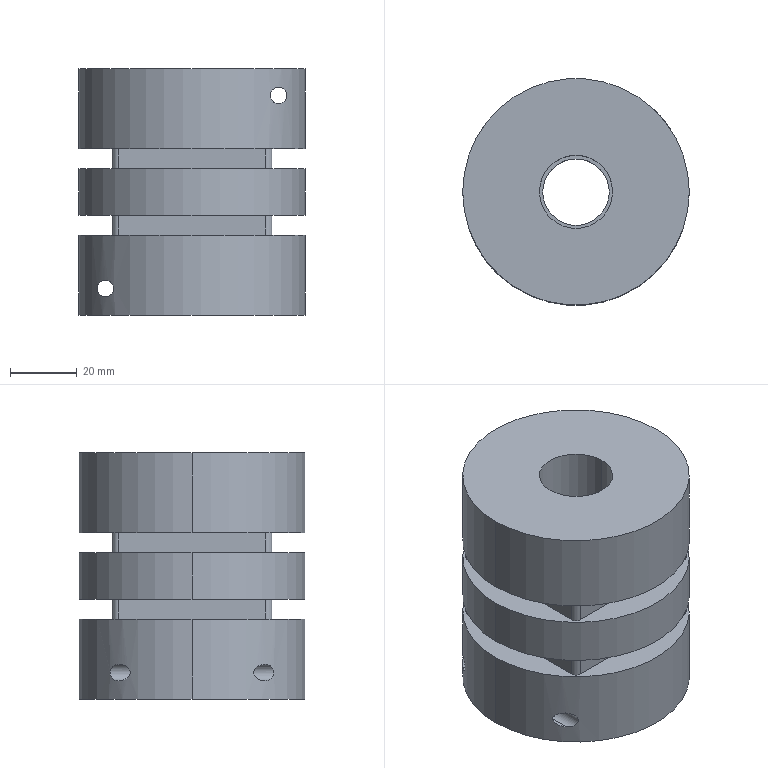Part | SolidWorks | features BaseBody 1 | 1 solid | 46 faces | box 68 x 68 x 74 mm | volume 205808 mm3 | cylinder 28 | plane 18 | commonest cylinder face diameters 4 x8 68 x6 5 x4 39 x4 20 x2 22 x2